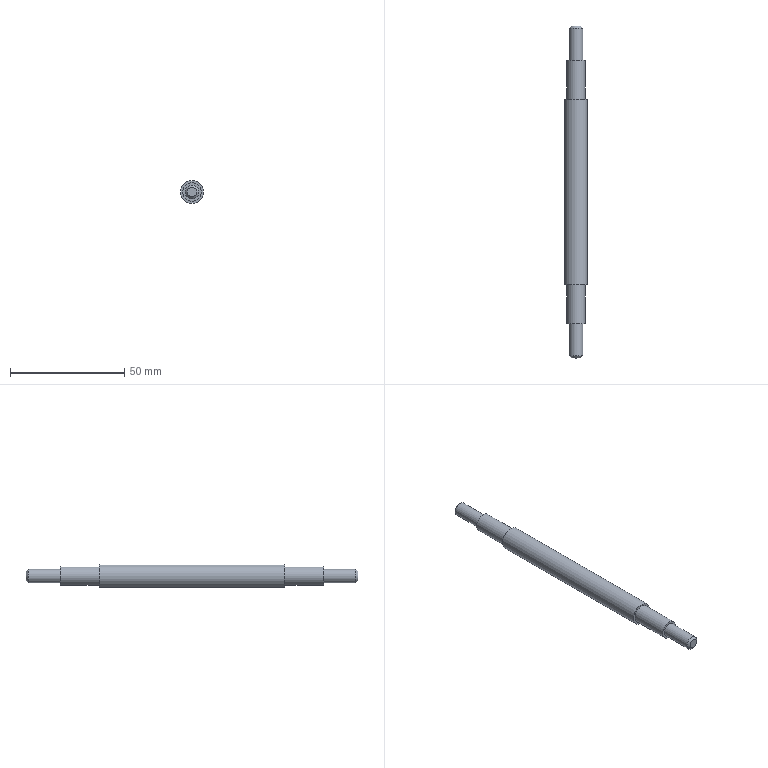Part | STEP file | 2-14.2 | 1 solid | 13 faces | box 10 x 145 x 10 mm | volume 8902 mm3 | plane 6 | cylinder 5 | cone 2 | commonest cylinder face diameters 6 x2 8 x2 10 x1
STEP:
#1=CARTESIAN_POINT('',(0.,0.,0.));
#2=DIRECTION('',(0.,0.,1.));
#3=DIRECTION('',(1.,0.,0.));
#4=AXIS2_PLACEMENT_3D('',#1,#2,#3);
#5=CARTESIAN_POINT('',(5.,-40.5,0.));
#6=VERTEX_POINT('',#5);
#7=CARTESIAN_POINT('',(5.,40.5,0.));
#8=VERTEX_POINT('',#7);
#9=CARTESIAN_POINT('',(5.,-40.5,0.));
#10=DIRECTION('',(0.,1.,0.));
#11=VECTOR('',#10,1.);
#12=LINE('',#9,#11);
#13=CARTESIAN_POINT('',(0.,-40.5,0.));
#14=DIRECTION('',(0.,1.,0.));
#15=DIRECTION('',(1.,0.,0.));
#16=AXIS2_PLACEMENT_3D('',#13,#14,#15);
#17=CYLINDRICAL_SURFACE('',#16,5.);
#18=CARTESIAN_POINT('',(6.283,0.));
#19=DIRECTION('',(0.,1.));
#20=VECTOR('',#19,1.);
#21=LINE('',#18,#20);
#22=(GEOMETRIC_REPRESENTATION_CONTEXT(2)PARAMETRIC_REPRESENTATION_CONTEXT()REPRESENTATION_CONTEXT('',''));
#23=DEFINITIONAL_REPRESENTATION('',(#21),#22);
#24=PCURVE('',#17,#23);
#25=CARTESIAN_POINT('',(0.,0.));
#26=DIRECTION('',(0.,1.));
#27=VECTOR('',#26,1.);
#28=LINE('',#25,#27);
#29=(GEOMETRIC_REPRESENTATION_CONTEXT(2)PARAMETRIC_REPRESENTATION_CONTEXT()REPRESENTATION_CONTEXT('',''));
#30=DEFINITIONAL_REPRESENTATION('',(#28),#29);
#31=PCURVE('',#17,#30);
#32=SEAM_CURVE('',#12,(#24,#31),.PCURVE_S1.);
#33=EDGE_CURVE('',#6,#8,#32,.T.);
#34=ORIENTED_EDGE('',*,*,#33,.T.);
#35=CARTESIAN_POINT('',(0.,40.5,0.));
#36=DIRECTION('',(0.,-1.,0.));
#37=DIRECTION('',(1.,0.,0.));
#38=AXIS2_PLACEMENT_3D('',#35,#36,#37);
#39=CIRCLE('',#38,5.);
#40=CARTESIAN_POINT('',(6.283,81.));
#41=DIRECTION('',(-1.,0.));
#42=VECTOR('',#41,1.);
#43=LINE('',#40,#42);
#44=(GEOMETRIC_REPRESENTATION_CONTEXT(2)PARAMETRIC_REPRESENTATION_CONTEXT()REPRESENTATION_CONTEXT('',''));
#45=DEFINITIONAL_REPRESENTATION('',(#43),#44);
#46=PCURVE('',#17,#45);
#47=CARTESIAN_POINT('',(-1.34,40.5,0.));
#48=DIRECTION('',(0.,-1.,0.));
#49=DIRECTION('',(1.,0.,0.));
#50=AXIS2_PLACEMENT_3D('',#47,#48,#49);
#51=PLANE('',#50);
#52=CARTESIAN_POINT('',(1.34,0.));
#53=DIRECTION('',(1.,0.));
#54=AXIS2_PLACEMENT_2D('',#52,#53);
#55=CIRCLE('',#54,5.);
#56=(GEOMETRIC_REPRESENTATION_CONTEXT(2)PARAMETRIC_REPRESENTATION_CONTEXT()REPRESENTATION_CONTEXT('',''));
#57=DEFINITIONAL_REPRESENTATION('',(#55),#56);
#58=PCURVE('',#51,#57);
#59=SURFACE_CURVE('',#39,(#46,#58),.PCURVE_S1.);
#60=EDGE_CURVE('',#8,#8,#59,.T.);
#61=ORIENTED_EDGE('',*,*,#60,.T.);
#62=ORIENTED_EDGE('',*,*,#33,.F.);
#63=CARTESIAN_POINT('',(0.,-40.5,0.));
#64=DIRECTION('',(0.,-1.,0.));
#65=DIRECTION('',(1.,0.,0.));
#66=AXIS2_PLACEMENT_3D('',#63,#64,#65);
#67=CIRCLE('',#66,5.);
#68=CARTESIAN_POINT('',(6.283,0.));
#69=DIRECTION('',(-1.,0.));
#70=VECTOR('',#69,1.);
#71=LINE('',#68,#70);
#72=(GEOMETRIC_REPRESENTATION_CONTEXT(2)PARAMETRIC_REPRESENTATION_CONTEXT()REPRESENTATION_CONTEXT('',''));
#73=DEFINITIONAL_REPRESENTATION('',(#71),#72);
#74=PCURVE('',#17,#73);
#75=CARTESIAN_POINT('',(-1.34,-40.5,0.));
#76=DIRECTION('',(0.,-1.,0.));
#77=DIRECTION('',(1.,0.,0.));
#78=AXIS2_PLACEMENT_3D('',#75,#76,#77);
#79=PLANE('',#78);
#80=CARTESIAN_POINT('',(1.34,0.));
#81=DIRECTION('',(1.,0.));
#82=AXIS2_PLACEMENT_2D('',#80,#81);
#83=CIRCLE('',#82,5.);
#84=(GEOMETRIC_REPRESENTATION_CONTEXT(2)PARAMETRIC_REPRESENTATION_CONTEXT()REPRESENTATION_CONTEXT('',''));
#85=DEFINITIONAL_REPRESENTATION('',(#83),#84);
#86=PCURVE('',#79,#85);
#87=SURFACE_CURVE('',#67,(#74,#86),.PCURVE_S1.);
#88=EDGE_CURVE('',#6,#6,#87,.T.);
#89=ORIENTED_EDGE('',*,*,#88,.F.);
#90=EDGE_LOOP('',(#34,#61,#62,#89));
#91=FACE_BOUND('',#90,.T.);
#92=ADVANCED_FACE('',(#91),#17,.T.);
#93=ORIENTED_EDGE('',*,*,#88,.T.);
#94=EDGE_LOOP('',(#93));
#95=FACE_BOUND('',#94,.T.);
#96=CARTESIAN_POINT('',(4.,-40.5,0.));
#97=VERTEX_POINT('',#96);
#98=CARTESIAN_POINT('',(0.,-40.5,0.));
#99=DIRECTION('',(0.,-1.,0.));
#100=DIRECTION('',(1.,0.,0.));
#101=AXIS2_PLACEMENT_3D('',#98,#99,#100);
#102=CIRCLE('',#101,4.);
#103=CARTESIAN_POINT('',(1.34,0.));
#104=DIRECTION('',(1.,0.));
#105=AXIS2_PLACEMENT_2D('',#103,#104);
#106=CIRCLE('',#105,4.);
#107=(GEOMETRIC_REPRESENTATION_CONTEXT(2)PARAMETRIC_REPRESENTATION_CONTEXT()REPRESENTATION_CONTEXT('',''));
#108=DEFINITIONAL_REPRESENTATION('',(#106),#107);
#109=PCURVE('',#79,#108);
#110=CARTESIAN_POINT('',(0.,-40.5,0.));
#111=DIRECTION('',(0.,-1.,0.));
#112=DIRECTION('',(1.,0.,0.));
#113=AXIS2_PLACEMENT_3D('',#110,#111,#112);
#114=CYLINDRICAL_SURFACE('',#113,4.);
#115=CARTESIAN_POINT('',(0.,0.));
#116=DIRECTION('',(1.,0.));
#117=VECTOR('',#116,1.);
#118=LINE('',#115,#117);
#119=(GEOMETRIC_REPRESENTATION_CONTEXT(2)PARAMETRIC_REPRESENTATION_CONTEXT()REPRESENTATION_CONTEXT('',''));
#120=DEFINITIONAL_REPRESENTATION('',(#118),#119);
#121=PCURVE('',#114,#120);
#122=SURFACE_CURVE('',#102,(#109,#121),.PCURVE_S1.);
#123=EDGE_CURVE('',#97,#97,#122,.T.);
#124=ORIENTED_EDGE('',*,*,#123,.F.);
#125=EDGE_LOOP('',(#124));
#126=FACE_BOUND('',#125,.T.);
#127=ADVANCED_FACE('',(#95,#126),#79,.T.);
#128=ORIENTED_EDGE('',*,*,#123,.T.);
#129=CARTESIAN_POINT('',(4.,-57.5,0.));
#130=VERTEX_POINT('',#129);
#131=CARTESIAN_POINT('',(4.,-40.5,0.));
#132=DIRECTION('',(0.,-1.,0.));
#133=VECTOR('',#132,1.);
#134=LINE('',#131,#133);
#135=CARTESIAN_POINT('',(6.283,0.));
#136=DIRECTION('',(0.,1.));
#137=VECTOR('',#136,1.);
#138=LINE('',#135,#137);
#139=(GEOMETRIC_REPRESENTATION_CONTEXT(2)PARAMETRIC_REPRESENTATION_CONTEXT()REPRESENTATION_CONTEXT('',''));
#140=DEFINITIONAL_REPRESENTATION('',(#138),#139);
#141=PCURVE('',#114,#140);
#142=CARTESIAN_POINT('',(0.,0.));
#143=DIRECTION('',(0.,1.));
#144=VECTOR('',#143,1.);
#145=LINE('',#142,#144);
#146=(GEOMETRIC_REPRESENTATION_CONTEXT(2)PARAMETRIC_REPRESENTATION_CONTEXT()REPRESENTATION_CONTEXT('',''));
#147=DEFINITIONAL_REPRESENTATION('',(#145),#146);
#148=PCURVE('',#114,#147);
#149=SEAM_CURVE('',#134,(#141,#148),.PCURVE_S1.);
#150=EDGE_CURVE('',#97,#130,#149,.T.);
#151=ORIENTED_EDGE('',*,*,#150,.T.);
#152=CARTESIAN_POINT('',(0.,-57.5,0.));
#153=DIRECTION('',(0.,-1.,0.));
#154=DIRECTION('',(1.,0.,0.));
#155=AXIS2_PLACEMENT_3D('',#152,#153,#154);
#156=CIRCLE('',#155,4.);
#157=CARTESIAN_POINT('',(0.,17.));
#158=DIRECTION('',(1.,0.));
#159=VECTOR('',#158,1.);
#160=LINE('',#157,#159);
#161=(GEOMETRIC_REPRESENTATION_CONTEXT(2)PARAMETRIC_REPRESENTATION_CONTEXT()REPRESENTATION_CONTEXT('',''));
#162=DEFINITIONAL_REPRESENTATION('',(#160),#161);
#163=PCURVE('',#114,#162);
#164=CARTESIAN_POINT('',(-1.072,-57.5,0.));
#165=DIRECTION('',(0.,-1.,0.));
#166=DIRECTION('',(1.,0.,0.));
#167=AXIS2_PLACEMENT_3D('',#164,#165,#166);
#168=PLANE('',#167);
#169=CARTESIAN_POINT('',(1.072,0.));
#170=DIRECTION('',(1.,0.));
#171=AXIS2_PLACEMENT_2D('',#169,#170);
#172=CIRCLE('',#171,4.);
#173=(GEOMETRIC_REPRESENTATION_CONTEXT(2)PARAMETRIC_REPRESENTATION_CONTEXT()REPRESENTATION_CONTEXT('',''));
#174=DEFINITIONAL_REPRESENTATION('',(#172),#173);
#175=PCURVE('',#168,#174);
#176=SURFACE_CURVE('',#156,(#163,#175),.PCURVE_S1.);
#177=EDGE_CURVE('',#130,#130,#176,.T.);
#178=ORIENTED_EDGE('',*,*,#177,.F.);
#179=ORIENTED_EDGE('',*,*,#150,.F.);
#180=EDGE_LOOP('',(#128,#151,#178,#179));
#181=FACE_BOUND('',#180,.T.);
#182=ADVANCED_FACE('',(#181),#114,.T.);
#183=ORIENTED_EDGE('',*,*,#177,.T.);
#184=EDGE_LOOP('',(#183));
#185=FACE_BOUND('',#184,.T.);
#186=CARTESIAN_POINT('',(3.,-57.5,0.));
#187=VERTEX_POINT('',#186);
#188=CARTESIAN_POINT('',(0.,-57.5,0.));
#189=DIRECTION('',(0.,-1.,0.));
#190=DIRECTION('',(1.,0.,0.));
#191=AXIS2_PLACEMENT_3D('',#188,#189,#190);
#192=CIRCLE('',#191,3.);
#193=CARTESIAN_POINT('',(1.072,0.));
#194=DIRECTION('',(1.,0.));
#195=AXIS2_PLACEMENT_2D('',#193,#194);
#196=CIRCLE('',#195,3.);
#197=(GEOMETRIC_REPRESENTATION_CONTEXT(2)PARAMETRIC_REPRESENTATION_CONTEXT()REPRESENTATION_CONTEXT('',''));
#198=DEFINITIONAL_REPRESENTATION('',(#196),#197);
#199=PCURVE('',#168,#198);
#200=CARTESIAN_POINT('',(0.,-57.5,0.));
#201=DIRECTION('',(0.,-1.,0.));
#202=DIRECTION('',(1.,0.,0.));
#203=AXIS2_PLACEMENT_3D('',#200,#201,#202);
#204=CYLINDRICAL_SURFACE('',#203,3.);
#205=CARTESIAN_POINT('',(0.,0.));
#206=DIRECTION('',(1.,0.));
#207=VECTOR('',#206,1.);
#208=LINE('',#205,#207);
#209=(GEOMETRIC_REPRESENTATION_CONTEXT(2)PARAMETRIC_REPRESENTATION_CONTEXT()REPRESENTATION_CONTEXT('',''));
#210=DEFINITIONAL_REPRESENTATION('',(#208),#209);
#211=PCURVE('',#204,#210);
#212=SURFACE_CURVE('',#192,(#199,#211),.PCURVE_S1.);
#213=EDGE_CURVE('',#187,#187,#212,.T.);
#214=ORIENTED_EDGE('',*,*,#213,.F.);
#215=EDGE_LOOP('',(#214));
#216=FACE_BOUND('',#215,.T.);
#217=ADVANCED_FACE('',(#185,#216),#168,.T.);
#218=ORIENTED_EDGE('',*,*,#60,.T.);
#219=EDGE_LOOP('',(#218));
#220=FACE_BOUND('',#219,.F.);
#221=CARTESIAN_POINT('',(4.,40.5,0.));
#222=VERTEX_POINT('',#221);
#223=CARTESIAN_POINT('',(0.,40.5,0.));
#224=DIRECTION('',(0.,-1.,0.));
#225=DIRECTION('',(1.,0.,0.));
#226=AXIS2_PLACEMENT_3D('',#223,#224,#225);
#227=CIRCLE('',#226,4.);
#228=CARTESIAN_POINT('',(1.34,0.));
#229=DIRECTION('',(1.,0.));
#230=AXIS2_PLACEMENT_2D('',#228,#229);
#231=CIRCLE('',#230,4.);
#232=(GEOMETRIC_REPRESENTATION_CONTEXT(2)PARAMETRIC_REPRESENTATION_CONTEXT()REPRESENTATION_CONTEXT('',''));
#233=DEFINITIONAL_REPRESENTATION('',(#231),#232);
#234=PCURVE('',#51,#233);
#235=CARTESIAN_POINT('',(0.,40.5,0.));
#236=DIRECTION('',(0.,1.,0.));
#237=DIRECTION('',(1.,0.,0.));
#238=AXIS2_PLACEMENT_3D('',#235,#236,#237);
#239=CYLINDRICAL_SURFACE('',#238,4.);
#240=CARTESIAN_POINT('',(6.283,0.));
#241=DIRECTION('',(-1.,0.));
#242=VECTOR('',#241,1.);
#243=LINE('',#240,#242);
#244=(GEOMETRIC_REPRESENTATION_CONTEXT(2)PARAMETRIC_REPRESENTATION_CONTEXT()REPRESENTATION_CONTEXT('',''));
#245=DEFINITIONAL_REPRESENTATION('',(#243),#244);
#246=PCURVE('',#239,#245);
#247=SURFACE_CURVE('',#227,(#234,#246),.PCURVE_S1.);
#248=EDGE_CURVE('',#222,#222,#247,.T.);
#249=ORIENTED_EDGE('',*,*,#248,.F.);
#250=EDGE_LOOP('',(#249));
#251=FACE_BOUND('',#250,.F.);
#252=ADVANCED_FACE('',(#220,#251),#51,.F.);
#253=CARTESIAN_POINT('',(4.,57.5,0.));
#254=VERTEX_POINT('',#253);
#255=CARTESIAN_POINT('',(4.,40.5,0.));
#256=DIRECTION('',(0.,1.,0.));
#257=VECTOR('',#256,1.);
#258=LINE('',#255,#257);
#259=CARTESIAN_POINT('',(6.283,0.));
#260=DIRECTION('',(0.,1.));
#261=VECTOR('',#260,1.);
#262=LINE('',#259,#261);
#263=(GEOMETRIC_REPRESENTATION_CONTEXT(2)PARAMETRIC_REPRESENTATION_CONTEXT()REPRESENTATION_CONTEXT('',''));
#264=DEFINITIONAL_REPRESENTATION('',(#262),#263);
#265=PCURVE('',#239,#264);
#266=CARTESIAN_POINT('',(0.,0.));
#267=DIRECTION('',(0.,1.));
#268=VECTOR('',#267,1.);
#269=LINE('',#266,#268);
#270=(GEOMETRIC_REPRESENTATION_CONTEXT(2)PARAMETRIC_REPRESENTATION_CONTEXT()REPRESENTATION_CONTEXT('',''));
#271=DEFINITIONAL_REPRESENTATION('',(#269),#270);
#272=PCURVE('',#239,#271);
#273=SEAM_CURVE('',#258,(#265,#272),.PCURVE_S1.);
#274=EDGE_CURVE('',#222,#254,#273,.T.);
#275=ORIENTED_EDGE('',*,*,#274,.T.);
#276=CARTESIAN_POINT('',(0.,57.5,0.));
#277=DIRECTION('',(0.,-1.,0.));
#278=DIRECTION('',(1.,0.,0.));
#279=AXIS2_PLACEMENT_3D('',#276,#277,#278);
#280=CIRCLE('',#279,4.);
#281=CARTESIAN_POINT('',(6.283,17.));
#282=DIRECTION('',(-1.,0.));
#283=VECTOR('',#282,1.);
#284=LINE('',#281,#283);
#285=(GEOMETRIC_REPRESENTATION_CONTEXT(2)PARAMETRIC_REPRESENTATION_CONTEXT()REPRESENTATION_CONTEXT('',''));
#286=DEFINITIONAL_REPRESENTATION('',(#284),#285);
#287=PCURVE('',#239,#286);
#288=CARTESIAN_POINT('',(-1.072,57.5,0.));
#289=DIRECTION('',(0.,-1.,0.));
#290=DIRECTION('',(1.,0.,0.));
#291=AXIS2_PLACEMENT_3D('',#288,#289,#290);
#292=PLANE('',#291);
#293=CARTESIAN_POINT('',(1.072,0.));
#294=DIRECTION('',(1.,0.));
#295=AXIS2_PLACEMENT_2D('',#293,#294);
#296=CIRCLE('',#295,4.);
#297=(GEOMETRIC_REPRESENTATION_CONTEXT(2)PARAMETRIC_REPRESENTATION_CONTEXT()REPRESENTATION_CONTEXT('',''));
#298=DEFINITIONAL_REPRESENTATION('',(#296),#297);
#299=PCURVE('',#292,#298);
#300=SURFACE_CURVE('',#280,(#287,#299),.PCURVE_S1.);
#301=EDGE_CURVE('',#254,#254,#300,.T.);
#302=ORIENTED_EDGE('',*,*,#301,.T.);
#303=ORIENTED_EDGE('',*,*,#274,.F.);
#304=ORIENTED_EDGE('',*,*,#248,.F.);
#305=EDGE_LOOP('',(#275,#302,#303,#304));
#306=FACE_BOUND('',#305,.T.);
#307=ADVANCED_FACE('',(#306),#239,.T.);
#308=ORIENTED_EDGE('',*,*,#301,.T.);
#309=EDGE_LOOP('',(#308));
#310=FACE_BOUND('',#309,.F.);
#311=CARTESIAN_POINT('',(3.,57.5,0.));
#312=VERTEX_POINT('',#311);
#313=CARTESIAN_POINT('',(0.,57.5,0.));
#314=DIRECTION('',(0.,-1.,0.));
#315=DIRECTION('',(1.,0.,0.));
#316=AXIS2_PLACEMENT_3D('',#313,#314,#315);
#317=CIRCLE('',#316,3.);
#318=CARTESIAN_POINT('',(1.072,0.));
#319=DIRECTION('',(1.,0.));
#320=AXIS2_PLACEMENT_2D('',#318,#319);
#321=CIRCLE('',#320,3.);
#322=(GEOMETRIC_REPRESENTATION_CONTEXT(2)PARAMETRIC_REPRESENTATION_CONTEXT()REPRESENTATION_CONTEXT('',''));
#323=DEFINITIONAL_REPRESENTATION('',(#321),#322);
#324=PCURVE('',#292,#323);
#325=CARTESIAN_POINT('',(0.,57.5,0.));
#326=DIRECTION('',(0.,1.,0.));
#327=DIRECTION('',(1.,0.,0.));
#328=AXIS2_PLACEMENT_3D('',#325,#326,#327);
#329=CYLINDRICAL_SURFACE('',#328,3.);
#330=CARTESIAN_POINT('',(6.283,0.));
#331=DIRECTION('',(-1.,0.));
#332=VECTOR('',#331,1.);
#333=LINE('',#330,#332);
#334=(GEOMETRIC_REPRESENTATION_CONTEXT(2)PARAMETRIC_REPRESENTATION_CONTEXT()REPRESENTATION_CONTEXT('',''));
#335=DEFINITIONAL_REPRESENTATION('',(#333),#334);
#336=PCURVE('',#329,#335);
#337=SURFACE_CURVE('',#317,(#324,#336),.PCURVE_S1.);
#338=EDGE_CURVE('',#312,#312,#337,.T.);
#339=ORIENTED_EDGE('',*,*,#338,.F.);
#340=EDGE_LOOP('',(#339));
#341=FACE_BOUND('',#340,.F.);
#342=ADVANCED_FACE('',(#310,#341),#292,.F.);
#343=ORIENTED_EDGE('',*,*,#213,.T.);
#344=CARTESIAN_POINT('',(3.,-71.5,0.));
#345=VERTEX_POINT('',#344);
#346=CARTESIAN_POINT('',(3.,-57.5,0.));
#347=DIRECTION('',(0.,-1.,0.));
#348=VECTOR('',#347,1.);
#349=LINE('',#346,#348);
#350=CARTESIAN_POINT('',(6.283,0.));
#351=DIRECTION('',(0.,1.));
#352=VECTOR('',#351,1.);
#353=LINE('',#350,#352);
#354=(GEOMETRIC_REPRESENTATION_CONTEXT(2)PARAMETRIC_REPRESENTATION_CONTEXT()REPRESENTATION_CONTEXT('',''));
#355=DEFINITIONAL_REPRESENTATION('',(#353),#354);
#356=PCURVE('',#204,#355);
#357=CARTESIAN_POINT('',(0.,0.));
#358=DIRECTION('',(0.,1.));
#359=VECTOR('',#358,1.);
#360=LINE('',#357,#359);
#361=(GEOMETRIC_REPRESENTATION_CONTEXT(2)PARAMETRIC_REPRESENTATION_CONTEXT()REPRESENTATION_CONTEXT('',''));
#362=DEFINITIONAL_REPRESENTATION('',(#360),#361);
#363=PCURVE('',#204,#362);
#364=SEAM_CURVE('',#349,(#356,#363),.PCURVE_S1.);
#365=EDGE_CURVE('',#187,#345,#364,.T.);
#366=ORIENTED_EDGE('',*,*,#365,.T.);
#367=CARTESIAN_POINT('',(0.,-71.5,0.));
#368=DIRECTION('',(0.,1.,0.));
#369=DIRECTION('',(1.,0.,0.));
#370=AXIS2_PLACEMENT_3D('',#367,#368,#369);
#371=CIRCLE('',#370,3.);
#372=CARTESIAN_POINT('',(6.283,14.));
#373=DIRECTION('',(-1.,0.));
#374=VECTOR('',#373,1.);
#375=LINE('',#372,#374);
#376=(GEOMETRIC_REPRESENTATION_CONTEXT(2)PARAMETRIC_REPRESENTATION_CONTEXT()REPRESENTATION_CONTEXT('',''));
#377=DEFINITIONAL_REPRESENTATION('',(#375),#376);
#378=PCURVE('',#204,#377);
#379=CARTESIAN_POINT('',(0.,-72.5,0.));
#380=DIRECTION('',(0.,1.,0.));
#381=DIRECTION('',(1.,0.,0.));
#382=AXIS2_PLACEMENT_3D('',#379,#380,#381);
#383=CONICAL_SURFACE('',#382,2.,0.7854);
#384=CARTESIAN_POINT('',(0.,1.));
#385=DIRECTION('',(1.,0.));
#386=VECTOR('',#385,1.);
#387=LINE('',#384,#386);
#388=(GEOMETRIC_REPRESENTATION_CONTEXT(2)PARAMETRIC_REPRESENTATION_CONTEXT()REPRESENTATION_CONTEXT('',''));
#389=DEFINITIONAL_REPRESENTATION('',(#387),#388);
#390=PCURVE('',#383,#389);
#391=SURFACE_CURVE('',#371,(#378,#390),.PCURVE_S1.);
#392=EDGE_CURVE('',#345,#345,#391,.T.);
#393=ORIENTED_EDGE('',*,*,#392,.T.);
#394=ORIENTED_EDGE('',*,*,#365,.F.);
#395=EDGE_LOOP('',(#343,#366,#393,#394));
#396=FACE_BOUND('',#395,.T.);
#397=ADVANCED_FACE('',(#396),#204,.T.);
#398=CARTESIAN_POINT('',(2.,-72.5,0.));
#399=VERTEX_POINT('',#398);
#400=CARTESIAN_POINT('',(0.,-72.5,0.));
#401=DIRECTION('',(0.,1.,0.));
#402=DIRECTION('',(1.,0.,0.));
#403=AXIS2_PLACEMENT_3D('',#400,#401,#402);
#404=CIRCLE('',#403,2.);
#405=CARTESIAN_POINT('',(-0.8038,-72.5,0.));
#406=DIRECTION('',(0.,-1.,0.));
#407=DIRECTION('',(1.,0.,0.));
#408=AXIS2_PLACEMENT_3D('',#405,#406,#407);
#409=PLANE('',#408);
#410=CARTESIAN_POINT('',(2.804,0.));
#411=CARTESIAN_POINT('',(2.804,-3.464));
#412=CARTESIAN_POINT('',(-0.1962,-1.732));
#413=CARTESIAN_POINT('',(-3.196,0.));
#414=CARTESIAN_POINT('',(-0.1962,1.732));
#415=CARTESIAN_POINT('',(2.804,3.464));
#416=CARTESIAN_POINT('',(2.804,0.));
#417=(BOUNDED_CURVE()B_SPLINE_CURVE(2,(#410,#411,#412,#413,#414,#415,#416),.UNSPECIFIED.,.T.,.F.)B_SPLINE_CURVE_WITH_KNOTS((1,2,2,2,2,1),(-2.094,0.,2.094,4.189,6.283,8.378),.UNSPECIFIED.)CURVE()GEOMETRIC_REPRESENTATION_ITEM()RATIONAL_B_SPLINE_CURVE((1.,0.5,1.,0.5,1.,0.5,1.))REPRESENTATION_ITEM(''));
#418=(GEOMETRIC_REPRESENTATION_CONTEXT(2)PARAMETRIC_REPRESENTATION_CONTEXT()REPRESENTATION_CONTEXT('',''));
#419=DEFINITIONAL_REPRESENTATION('',(#417),#418);
#420=PCURVE('',#409,#419);
#421=CARTESIAN_POINT('',(0.,0.));
#422=DIRECTION('',(1.,0.));
#423=VECTOR('',#422,1.);
#424=LINE('',#421,#423);
#425=(GEOMETRIC_REPRESENTATION_CONTEXT(2)PARAMETRIC_REPRESENTATION_CONTEXT()REPRESENTATION_CONTEXT('',''));
#426=DEFINITIONAL_REPRESENTATION('',(#424),#425);
#427=PCURVE('',#383,#426);
#428=SURFACE_CURVE('',#404,(#420,#427),.PCURVE_S1.);
#429=EDGE_CURVE('',#399,#399,#428,.T.);
#430=ORIENTED_EDGE('',*,*,#429,.F.);
#431=EDGE_LOOP('',(#430));
#432=FACE_BOUND('',#431,.T.);
#433=ADVANCED_FACE('',(#432),#409,.T.);
#434=CARTESIAN_POINT('',(3.,71.5,0.));
#435=VERTEX_POINT('',#434);
#436=CARTESIAN_POINT('',(3.,57.5,0.));
#437=DIRECTION('',(0.,1.,0.));
#438=VECTOR('',#437,1.);
#439=LINE('',#436,#438);
#440=CARTESIAN_POINT('',(6.283,0.));
#441=DIRECTION('',(0.,1.));
#442=VECTOR('',#441,1.);
#443=LINE('',#440,#442);
#444=(GEOMETRIC_REPRESENTATION_CONTEXT(2)PARAMETRIC_REPRESENTATION_CONTEXT()REPRESENTATION_CONTEXT('',''));
#445=DEFINITIONAL_REPRESENTATION('',(#443),#444);
#446=PCURVE('',#329,#445);
#447=CARTESIAN_POINT('',(0.,0.));
#448=DIRECTION('',(0.,1.));
#449=VECTOR('',#448,1.);
#450=LINE('',#447,#449);
#451=(GEOMETRIC_REPRESENTATION_CONTEXT(2)PARAMETRIC_REPRESENTATION_CONTEXT()REPRESENTATION_CONTEXT('',''));
#452=DEFINITIONAL_REPRESENTATION('',(#450),#451);
#453=PCURVE('',#329,#452);
#454=SEAM_CURVE('',#439,(#446,#453),.PCURVE_S1.);
#455=EDGE_CURVE('',#312,#435,#454,.T.);
#456=ORIENTED_EDGE('',*,*,#455,.T.);
#457=CARTESIAN_POINT('',(0.,71.5,0.));
#458=DIRECTION('',(0.,-1.,0.));
#459=DIRECTION('',(1.,0.,0.));
#460=AXIS2_PLACEMENT_3D('',#457,#458,#459);
#461=CIRCLE('',#460,3.);
#462=CARTESIAN_POINT('',(6.283,14.));
#463=DIRECTION('',(-1.,0.));
#464=VECTOR('',#463,1.);
#465=LINE('',#462,#464);
#466=(GEOMETRIC_REPRESENTATION_CONTEXT(2)PARAMETRIC_REPRESENTATION_CONTEXT()REPRESENTATION_CONTEXT('',''));
#467=DEFINITIONAL_REPRESENTATION('',(#465),#466);
#468=PCURVE('',#329,#467);
#469=CARTESIAN_POINT('',(0.,72.5,0.));
#470=DIRECTION('',(0.,-1.,0.));
#471=DIRECTION('',(1.,0.,0.));
#472=AXIS2_PLACEMENT_3D('',#469,#470,#471);
#473=CONICAL_SURFACE('',#472,2.,0.7854);
#474=CARTESIAN_POINT('',(0.,1.));
#475=DIRECTION('',(1.,0.));
#476=VECTOR('',#475,1.);
#477=LINE('',#474,#476);
#478=(GEOMETRIC_REPRESENTATION_CONTEXT(2)PARAMETRIC_REPRESENTATION_CONTEXT()REPRESENTATION_CONTEXT('',''));
#479=DEFINITIONAL_REPRESENTATION('',(#477),#478);
#480=PCURVE('',#473,#479);
#481=SURFACE_CURVE('',#461,(#468,#480),.PCURVE_S1.);
#482=EDGE_CURVE('',#435,#435,#481,.T.);
#483=ORIENTED_EDGE('',*,*,#482,.T.);
#484=ORIENTED_EDGE('',*,*,#455,.F.);
#485=ORIENTED_EDGE('',*,*,#338,.F.);
#486=EDGE_LOOP('',(#456,#483,#484,#485));
#487=FACE_BOUND('',#486,.T.);
#488=ADVANCED_FACE('',(#487),#329,.T.);
#489=CARTESIAN_POINT('',(2.,72.5,0.));
#490=VERTEX_POINT('',#489);
#491=CARTESIAN_POINT('',(0.,72.5,0.));
#492=DIRECTION('',(0.,-1.,0.));
#493=DIRECTION('',(1.,0.,0.));
#494=AXIS2_PLACEMENT_3D('',#491,#492,#493);
#495=CIRCLE('',#494,2.);
#496=CARTESIAN_POINT('',(-0.8038,72.5,0.));
#497=DIRECTION('',(0.,-1.,0.));
#498=DIRECTION('',(1.,0.,0.));
#499=AXIS2_PLACEMENT_3D('',#496,#497,#498);
#500=PLANE('',#499);
#501=CARTESIAN_POINT('',(0.8038,0.));
#502=DIRECTION('',(1.,0.));
#503=AXIS2_PLACEMENT_2D('',#501,#502);
#504=CIRCLE('',#503,2.);
#505=(GEOMETRIC_REPRESENTATION_CONTEXT(2)PARAMETRIC_REPRESENTATION_CONTEXT()REPRESENTATION_CONTEXT('',''));
#506=DEFINITIONAL_REPRESENTATION('',(#504),#505);
#507=PCURVE('',#500,#506);
#508=CARTESIAN_POINT('',(0.,0.));
#509=DIRECTION('',(1.,0.));
#510=VECTOR('',#509,1.);
#511=LINE('',#508,#510);
#512=(GEOMETRIC_REPRESENTATION_CONTEXT(2)PARAMETRIC_REPRESENTATION_CONTEXT()REPRESENTATION_CONTEXT('',''));
#513=DEFINITIONAL_REPRESENTATION('',(#511),#512);
#514=PCURVE('',#473,#513);
#515=SURFACE_CURVE('',#495,(#507,#514),.PCURVE_S1.);
#516=EDGE_CURVE('',#490,#490,#515,.T.);
#517=ORIENTED_EDGE('',*,*,#516,.T.);
#518=EDGE_LOOP('',(#517));
#519=FACE_BOUND('',#518,.F.);
#520=ADVANCED_FACE('',(#519),#500,.F.);
#521=CARTESIAN_POINT('',(2.,-72.5,0.));
#522=DIRECTION('',(0.7071,0.7071,0.));
#523=VECTOR('',#522,1.);
#524=LINE('',#521,#523);
#525=CARTESIAN_POINT('',(6.283,0.));
#526=DIRECTION('',(0.,1.));
#527=VECTOR('',#526,1.);
#528=LINE('',#525,#527);
#529=(GEOMETRIC_REPRESENTATION_CONTEXT(2)PARAMETRIC_REPRESENTATION_CONTEXT()REPRESENTATION_CONTEXT('',''));
#530=DEFINITIONAL_REPRESENTATION('',(#528),#529);
#531=PCURVE('',#383,#530);
#532=CARTESIAN_POINT('',(0.,0.));
#533=DIRECTION('',(0.,1.));
#534=VECTOR('',#533,1.);
#535=LINE('',#532,#534);
#536=(GEOMETRIC_REPRESENTATION_CONTEXT(2)PARAMETRIC_REPRESENTATION_CONTEXT()REPRESENTATION_CONTEXT('',''));
#537=DEFINITIONAL_REPRESENTATION('',(#535),#536);
#538=PCURVE('',#383,#537);
#539=SEAM_CURVE('',#524,(#531,#538),.PCURVE_S1.);
#540=EDGE_CURVE('',#399,#345,#539,.T.);
#541=ORIENTED_EDGE('',*,*,#540,.T.);
#542=ORIENTED_EDGE('',*,*,#392,.F.);
#543=ORIENTED_EDGE('',*,*,#540,.F.);
#544=ORIENTED_EDGE('',*,*,#429,.T.);
#545=EDGE_LOOP('',(#541,#542,#543,#544));
#546=FACE_BOUND('',#545,.T.);
#547=ADVANCED_FACE('',(#546),#383,.T.);
#548=CARTESIAN_POINT('',(2.,72.5,0.));
#549=DIRECTION('',(0.7071,-0.7071,0.));
#550=VECTOR('',#549,1.);
#551=LINE('',#548,#550);
#552=CARTESIAN_POINT('',(6.283,0.));
#553=DIRECTION('',(0.,1.));
#554=VECTOR('',#553,1.);
#555=LINE('',#552,#554);
#556=(GEOMETRIC_REPRESENTATION_CONTEXT(2)PARAMETRIC_REPRESENTATION_CONTEXT()REPRESENTATION_CONTEXT('',''));
#557=DEFINITIONAL_REPRESENTATION('',(#555),#556);
#558=PCURVE('',#473,#557);
#559=CARTESIAN_POINT('',(0.,0.));
#560=DIRECTION('',(0.,1.));
#561=VECTOR('',#560,1.);
#562=LINE('',#559,#561);
#563=(GEOMETRIC_REPRESENTATION_CONTEXT(2)PARAMETRIC_REPRESENTATION_CONTEXT()REPRESENTATION_CONTEXT('',''));
#564=DEFINITIONAL_REPRESENTATION('',(#562),#563);
#565=PCURVE('',#473,#564);
#566=SEAM_CURVE('',#551,(#558,#565),.PCURVE_S1.);
#567=EDGE_CURVE('',#490,#435,#566,.T.);
#568=ORIENTED_EDGE('',*,*,#567,.T.);
#569=ORIENTED_EDGE('',*,*,#482,.F.);
#570=ORIENTED_EDGE('',*,*,#567,.F.);
#571=ORIENTED_EDGE('',*,*,#516,.T.);
#572=EDGE_LOOP('',(#568,#569,#570,#571));
#573=FACE_BOUND('',#572,.T.);
#574=ADVANCED_FACE('',(#573),#473,.T.);
#575=CLOSED_SHELL('',(#92,#127,#182,#217,#252,#307,#342,#397,#433,#488,#520,#547,#574));
#576=MANIFOLD_SOLID_BREP('',#575);
#577=(LENGTH_UNIT()NAMED_UNIT(*)SI_UNIT(.MILLI.,.METRE.));
#578=UNCERTAINTY_MEASURE_WITH_UNIT(LENGTH_MEASURE(0.0000001),#577,'','');
#579=(NAMED_UNIT(*)PLANE_ANGLE_UNIT()SI_UNIT($,.RADIAN.));
#580=(NAMED_UNIT(*)SI_UNIT($,.STERADIAN.)SOLID_ANGLE_UNIT());
#581=(GEOMETRIC_REPRESENTATION_CONTEXT(3)GLOBAL_UNCERTAINTY_ASSIGNED_CONTEXT((#578))GLOBAL_UNIT_ASSIGNED_CONTEXT((#577,#579,#580))REPRESENTATION_CONTEXT('',''));
#582=ADVANCED_BREP_SHAPE_REPRESENTATION('',(#4,#576),#581);